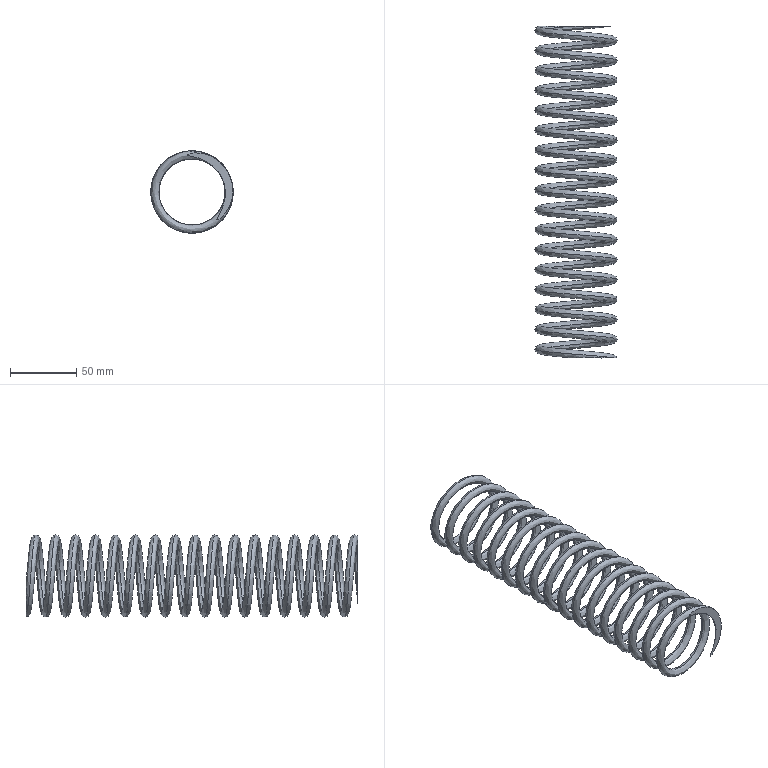Part | SolidWorks | features Helix 1, ICE 1, RefAxis 1, Sweep 1 | 1 solid | 4 faces | box 62 x 250 x 62 mm | volume 81996 mm3 | spline 2 | plane 2